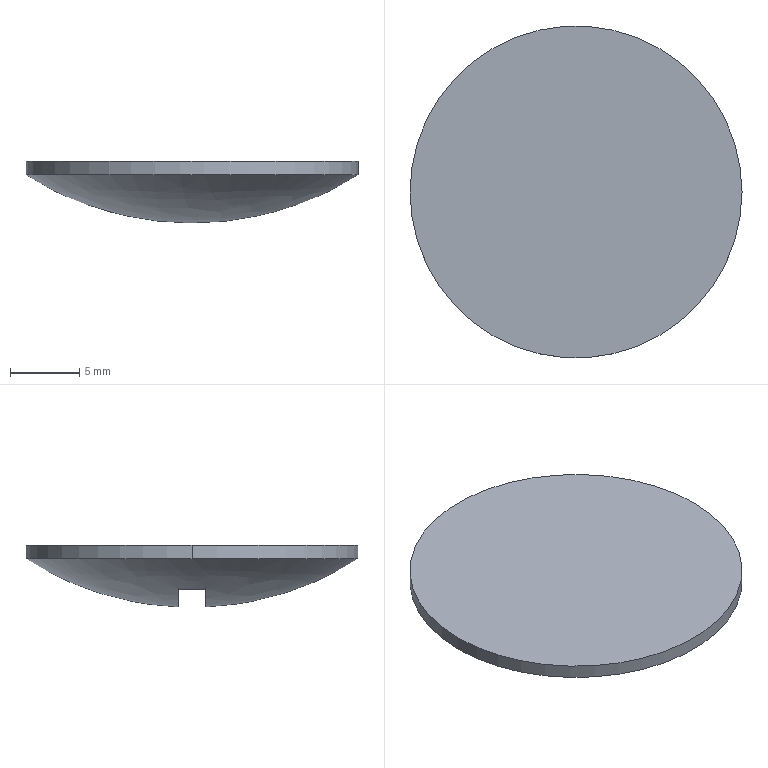Part | STEP file | PRODUCT_NAME_42_default | 1 solid | 9 faces | box 24 x 24 x 4.478 mm | volume 1175 mm3 | plane 6 | cylinder 2 | spline 1 | commonest cylinder face diameters 24 x2
STEP:
#1=CARTESIAN_POINT('',(0.,0.,0.));
#2=DIRECTION('',(0.,0.,1.));
#3=DIRECTION('',(1.,0.,0.));
#4=AXIS2_PLACEMENT_3D('',#1,#2,#3);
#5=CARTESIAN_POINT('',(194.5,-10.5,-47.5));
#6=VERTEX_POINT('',#5);
#7=CARTESIAN_POINT('',(170.5,-10.5,-47.5));
#8=VERTEX_POINT('',#7);
#9=CARTESIAN_POINT('',(182.5,-10.5,-47.5));
#10=DIRECTION('',(0.,0.,1.));
#11=DIRECTION('',(-1.,0.,0.));
#12=AXIS2_PLACEMENT_3D('',#9,#10,#11);
#13=CIRCLE('',#12,12.);
#14=CARTESIAN_POINT('',(182.5,-10.5,-48.));
#15=DIRECTION('',(0.,0.,-1.));
#16=DIRECTION('',(-1.,0.,0.));
#17=AXIS2_PLACEMENT_3D('',#14,#15,#16);
#18=CYLINDRICAL_SURFACE('',#17,12.);
#19=CARTESIAN_POINT('',(6.283,-0.5));
#20=DIRECTION('',(-1.,0.));
#21=VECTOR('',#20,1.);
#22=LINE('',#19,#21);
#23=(GEOMETRIC_REPRESENTATION_CONTEXT(2)PARAMETRIC_REPRESENTATION_CONTEXT()REPRESENTATION_CONTEXT('',''));
#24=DEFINITIONAL_REPRESENTATION('',(#22),#23);
#25=PCURVE('',#18,#24);
#26=CARTESIAN_POINT('',(188.5,-10.5,-47.5));
#27=DIRECTION('',(0.,0.,1.));
#28=DIRECTION('',(1.,0.,0.));
#29=AXIS2_PLACEMENT_3D('',#26,#27,#28);
#30=PLANE('',#29);
#31=CARTESIAN_POINT('',(-6.,0.));
#32=DIRECTION('',(-1.,0.));
#33=AXIS2_PLACEMENT_2D('',#31,#32);
#34=CIRCLE('',#33,12.);
#35=(GEOMETRIC_REPRESENTATION_CONTEXT(2)PARAMETRIC_REPRESENTATION_CONTEXT()REPRESENTATION_CONTEXT('',''));
#36=DEFINITIONAL_REPRESENTATION('',(#34),#35);
#37=PCURVE('',#30,#36);
#38=SURFACE_CURVE('',#13,(#25,#37),.PCURVE_S1.);
#39=EDGE_CURVE('',#6,#8,#38,.T.);
#40=ORIENTED_EDGE('',*,*,#39,.F.);
#41=CARTESIAN_POINT('',(194.5,-10.5,-48.5));
#42=VERTEX_POINT('',#41);
#43=CARTESIAN_POINT('',(194.5,-10.5,-48.));
#44=DIRECTION('',(0.,0.,-1.));
#45=VECTOR('',#44,1.);
#46=LINE('',#43,#45);
#47=CARTESIAN_POINT('',(3.142,0.));
#48=DIRECTION('',(0.,1.));
#49=VECTOR('',#48,1.);
#50=LINE('',#47,#49);
#51=(GEOMETRIC_REPRESENTATION_CONTEXT(2)PARAMETRIC_REPRESENTATION_CONTEXT()REPRESENTATION_CONTEXT('',''));
#52=DEFINITIONAL_REPRESENTATION('',(#50),#51);
#53=PCURVE('',#18,#52);
#54=CARTESIAN_POINT('',(182.5,-10.5,-48.));
#55=DIRECTION('',(0.,0.,-1.));
#56=DIRECTION('',(-1.,0.,0.));
#57=AXIS2_PLACEMENT_3D('',#54,#55,#56);
#58=CYLINDRICAL_SURFACE('',#57,12.);
#59=CARTESIAN_POINT('',(3.142,0.));
#60=DIRECTION('',(0.,1.));
#61=VECTOR('',#60,1.);
#62=LINE('',#59,#61);
#63=(GEOMETRIC_REPRESENTATION_CONTEXT(2)PARAMETRIC_REPRESENTATION_CONTEXT()REPRESENTATION_CONTEXT('',''));
#64=DEFINITIONAL_REPRESENTATION('',(#62),#63);
#65=PCURVE('',#58,#64);
#66=SURFACE_CURVE('',#46,(#53,#65),.PCURVE_S1.);
#67=EDGE_CURVE('',#6,#42,#66,.T.);
#68=ORIENTED_EDGE('',*,*,#67,.T.);
#69=CARTESIAN_POINT('',(170.5,-10.5,-48.5));
#70=VERTEX_POINT('',#69);
#71=CARTESIAN_POINT('',(182.5,-10.5,-48.5));
#72=DIRECTION('',(0.,0.,1.));
#73=DIRECTION('',(-1.,0.,0.));
#74=AXIS2_PLACEMENT_3D('',#71,#72,#73);
#75=CIRCLE('',#74,12.);
#76=CARTESIAN_POINT('',(6.283,0.5));
#77=DIRECTION('',(-1.,0.));
#78=VECTOR('',#77,1.);
#79=LINE('',#76,#78);
#80=(GEOMETRIC_REPRESENTATION_CONTEXT(2)PARAMETRIC_REPRESENTATION_CONTEXT()REPRESENTATION_CONTEXT('',''));
#81=DEFINITIONAL_REPRESENTATION('',(#79),#80);
#82=PCURVE('',#18,#81);
#83=CARTESIAN_POINT('',(194.7,-20.681,-45.355));
#84=CARTESIAN_POINT('',(194.7,-14.291,-49.505));
#85=CARTESIAN_POINT('',(194.7,-6.671,-49.498));
#86=CARTESIAN_POINT('',(194.7,-0.2882,-45.335));
#87=CARTESIAN_POINT('',(187.09,-23.387,-49.521));
#88=CARTESIAN_POINT('',(187.09,-15.298,-54.774));
#89=CARTESIAN_POINT('',(187.09,-5.653,-54.765));
#90=CARTESIAN_POINT('',(187.09,2.426,-49.495));
#91=CARTESIAN_POINT('',(178.001,-23.396,-49.535));
#92=CARTESIAN_POINT('',(178.001,-15.301,-54.793));
#93=CARTESIAN_POINT('',(178.001,-5.649,-54.783));
#94=CARTESIAN_POINT('',(178.001,2.435,-49.51));
#95=CARTESIAN_POINT('',(170.372,-20.706,-45.394));
#96=CARTESIAN_POINT('',(170.372,-14.3,-49.555));
#97=CARTESIAN_POINT('',(170.372,-6.661,-49.547));
#98=CARTESIAN_POINT('',(170.372,-0.2627,-45.374));
#99=(BOUNDED_SURFACE()B_SPLINE_SURFACE(3,3,((#83,#84,#85,#86),(#87,#88,#89,#90),(#91,#92,#93,#94),(#95,#96,#97,#98)),.UNSPECIFIED.,.F.,.F.,.F.)B_SPLINE_SURFACE_WITH_KNOTS((4,4),(4,4),(0.,1.),(0.,1.),.PIECEWISE_BEZIER_KNOTS.)GEOMETRIC_REPRESENTATION_ITEM()RATIONAL_B_SPLINE_SURFACE(((1.,0.8921,0.8921,1.),(0.8923,0.796,0.796,0.8923),(0.8923,0.796,0.796,0.8923),(1.,0.8921,0.8921,1.)))REPRESENTATION_ITEM('')SURFACE());
#100=CARTESIAN_POINT('',(0.009777,0.4992));
#101=CARTESIAN_POINT('',(0.009731,0.5248));
#102=CARTESIAN_POINT('',(0.01378,0.5759));
#103=CARTESIAN_POINT('',(0.03134,0.6501));
#104=CARTESIAN_POINT('',(0.05961,0.7196));
#105=CARTESIAN_POINT('',(0.09719,0.7826));
#106=CARTESIAN_POINT('',(0.1425,0.8381));
#107=CARTESIAN_POINT('',(0.1941,0.8853));
#108=CARTESIAN_POINT('',(0.2505,0.9239));
#109=CARTESIAN_POINT('',(0.3105,0.9538));
#110=CARTESIAN_POINT('',(0.3729,0.975));
#111=CARTESIAN_POINT('',(0.4369,0.9877));
#112=CARTESIAN_POINT('',(0.5016,0.9919));
#113=CARTESIAN_POINT('',(0.5664,0.9877));
#114=CARTESIAN_POINT('',(0.6304,0.975));
#115=CARTESIAN_POINT('',(0.6928,0.9538));
#116=CARTESIAN_POINT('',(0.7528,0.9239));
#117=CARTESIAN_POINT('',(0.8092,0.8853));
#118=CARTESIAN_POINT('',(0.8608,0.8381));
#119=CARTESIAN_POINT('',(0.9062,0.7826));
#120=CARTESIAN_POINT('',(0.9439,0.7196));
#121=CARTESIAN_POINT('',(0.9722,0.6501));
#122=CARTESIAN_POINT('',(0.9897,0.5759));
#123=CARTESIAN_POINT('',(0.9938,0.5248));
#124=CARTESIAN_POINT('',(0.9937,0.4992));
#125=B_SPLINE_CURVE_WITH_KNOTS('',3,(#100,#101,#102,#103,#104,#105,#106,#107,#108,#109,#110,#111,#112,#113,#114,#115,#116,#117,#118,#119,#120,#121,#122,#123,#124),.UNSPECIFIED.,.F.,.F.,(4,1,1,1,1,1,1,1,1,1,1,1,1,1,1,1,1,1,1,1,1,1,4),(3.142,3.284,3.427,3.57,3.713,3.856,3.998,4.141,4.284,4.427,4.57,4.712,4.855,4.998,5.141,5.284,5.426,5.569,5.712,5.855,5.998,6.14,6.283),.QUASI_UNIFORM_KNOTS.);
#126=(GEOMETRIC_REPRESENTATION_CONTEXT(2)PARAMETRIC_REPRESENTATION_CONTEXT()REPRESENTATION_CONTEXT('',''));
#127=DEFINITIONAL_REPRESENTATION('',(#125),#126);
#128=PCURVE('',#99,#127);
#129=SURFACE_CURVE('',#75,(#82,#128),.PCURVE_S1.);
#130=EDGE_CURVE('',#42,#70,#129,.T.);
#131=ORIENTED_EDGE('',*,*,#130,.T.);
#132=CARTESIAN_POINT('',(170.5,-10.5,-48.));
#133=DIRECTION('',(0.,0.,-1.));
#134=VECTOR('',#133,1.);
#135=LINE('',#132,#134);
#136=CARTESIAN_POINT('',(0.,0.));
#137=DIRECTION('',(0.,1.));
#138=VECTOR('',#137,1.);
#139=LINE('',#136,#138);
#140=(GEOMETRIC_REPRESENTATION_CONTEXT(2)PARAMETRIC_REPRESENTATION_CONTEXT()REPRESENTATION_CONTEXT('',''));
#141=DEFINITIONAL_REPRESENTATION('',(#139),#140);
#142=PCURVE('',#18,#141);
#143=CARTESIAN_POINT('',(6.283,0.));
#144=DIRECTION('',(0.,1.));
#145=VECTOR('',#144,1.);
#146=LINE('',#143,#145);
#147=(GEOMETRIC_REPRESENTATION_CONTEXT(2)PARAMETRIC_REPRESENTATION_CONTEXT()REPRESENTATION_CONTEXT('',''));
#148=DEFINITIONAL_REPRESENTATION('',(#146),#147);
#149=PCURVE('',#58,#148);
#150=SURFACE_CURVE('',#135,(#142,#149),.PCURVE_S1.);
#151=EDGE_CURVE('',#8,#70,#150,.T.);
#152=ORIENTED_EDGE('',*,*,#151,.F.);
#153=EDGE_LOOP('',(#40,#68,#131,#152));
#154=FACE_BOUND('',#153,.T.);
#155=ADVANCED_FACE('',(#154),#18,.T.);
#156=CARTESIAN_POINT('',(182.5,-10.5,-47.5));
#157=DIRECTION('',(0.,0.,1.));
#158=DIRECTION('',(-1.,0.,0.));
#159=AXIS2_PLACEMENT_3D('',#156,#157,#158);
#160=CIRCLE('',#159,12.);
#161=CARTESIAN_POINT('',(-6.,0.));
#162=DIRECTION('',(-1.,0.));
#163=AXIS2_PLACEMENT_2D('',#161,#162);
#164=CIRCLE('',#163,12.);
#165=(GEOMETRIC_REPRESENTATION_CONTEXT(2)PARAMETRIC_REPRESENTATION_CONTEXT()REPRESENTATION_CONTEXT('',''));
#166=DEFINITIONAL_REPRESENTATION('',(#164),#165);
#167=PCURVE('',#30,#166);
#168=CARTESIAN_POINT('',(6.283,-0.5));
#169=DIRECTION('',(-1.,0.));
#170=VECTOR('',#169,1.);
#171=LINE('',#168,#170);
#172=(GEOMETRIC_REPRESENTATION_CONTEXT(2)PARAMETRIC_REPRESENTATION_CONTEXT()REPRESENTATION_CONTEXT('',''));
#173=DEFINITIONAL_REPRESENTATION('',(#171),#172);
#174=PCURVE('',#58,#173);
#175=SURFACE_CURVE('',#160,(#167,#174),.PCURVE_S1.);
#176=EDGE_CURVE('',#8,#6,#175,.T.);
#177=ORIENTED_EDGE('',*,*,#176,.T.);
#178=ORIENTED_EDGE('',*,*,#39,.T.);
#179=EDGE_LOOP('',(#177,#178));
#180=FACE_BOUND('',#179,.T.);
#181=ADVANCED_FACE('',(#180),#30,.T.);
#182=ORIENTED_EDGE('',*,*,#67,.F.);
#183=ORIENTED_EDGE('',*,*,#176,.F.);
#184=ORIENTED_EDGE('',*,*,#151,.T.);
#185=CARTESIAN_POINT('',(182.5,-10.5,-48.5));
#186=DIRECTION('',(0.,0.,1.));
#187=DIRECTION('',(-1.,0.,0.));
#188=AXIS2_PLACEMENT_3D('',#185,#186,#187);
#189=CIRCLE('',#188,12.);
#190=CARTESIAN_POINT('',(6.283,0.5));
#191=DIRECTION('',(-1.,0.));
#192=VECTOR('',#191,1.);
#193=LINE('',#190,#192);
#194=(GEOMETRIC_REPRESENTATION_CONTEXT(2)PARAMETRIC_REPRESENTATION_CONTEXT()REPRESENTATION_CONTEXT('',''));
#195=DEFINITIONAL_REPRESENTATION('',(#193),#194);
#196=PCURVE('',#58,#195);
#197=CARTESIAN_POINT('',(0.9937,0.4992));
#198=CARTESIAN_POINT('',(0.9938,0.4736));
#199=CARTESIAN_POINT('',(0.9897,0.4225));
#200=CARTESIAN_POINT('',(0.9722,0.3483));
#201=CARTESIAN_POINT('',(0.9439,0.2788));
#202=CARTESIAN_POINT('',(0.9062,0.2157));
#203=CARTESIAN_POINT('',(0.8608,0.1602));
#204=CARTESIAN_POINT('',(0.8092,0.1129));
#205=CARTESIAN_POINT('',(0.7528,0.07436));
#206=CARTESIAN_POINT('',(0.6928,0.04446));
#207=CARTESIAN_POINT('',(0.6304,0.02321));
#208=CARTESIAN_POINT('',(0.5664,0.01051));
#209=CARTESIAN_POINT('',(0.5016,0.006284));
#210=CARTESIAN_POINT('',(0.4369,0.01051));
#211=CARTESIAN_POINT('',(0.3729,0.02321));
#212=CARTESIAN_POINT('',(0.3105,0.04446));
#213=CARTESIAN_POINT('',(0.2505,0.07436));
#214=CARTESIAN_POINT('',(0.1941,0.1129));
#215=CARTESIAN_POINT('',(0.1425,0.1602));
#216=CARTESIAN_POINT('',(0.09719,0.2157));
#217=CARTESIAN_POINT('',(0.05961,0.2788));
#218=CARTESIAN_POINT('',(0.03134,0.3483));
#219=CARTESIAN_POINT('',(0.01378,0.4225));
#220=CARTESIAN_POINT('',(0.009731,0.4736));
#221=CARTESIAN_POINT('',(0.009777,0.4992));
#222=B_SPLINE_CURVE_WITH_KNOTS('',3,(#197,#198,#199,#200,#201,#202,#203,#204,#205,#206,#207,#208,#209,#210,#211,#212,#213,#214,#215,#216,#217,#218,#219,#220,#221),.UNSPECIFIED.,.F.,.F.,(4,1,1,1,1,1,1,1,1,1,1,1,1,1,1,1,1,1,1,1,1,1,4),(0.,0.1428,0.2856,0.4284,0.5712,0.714,0.8568,0.9996,1.142,1.285,1.428,1.571,1.714,1.856,1.999,2.142,2.285,2.428,2.57,2.713,2.856,2.999,3.142),.QUASI_UNIFORM_KNOTS.);
#223=(GEOMETRIC_REPRESENTATION_CONTEXT(2)PARAMETRIC_REPRESENTATION_CONTEXT()REPRESENTATION_CONTEXT('',''));
#224=DEFINITIONAL_REPRESENTATION('',(#222),#223);
#225=PCURVE('',#99,#224);
#226=SURFACE_CURVE('',#189,(#196,#225),.PCURVE_S1.);
#227=EDGE_CURVE('',#70,#42,#226,.T.);
#228=ORIENTED_EDGE('',*,*,#227,.T.);
#229=EDGE_LOOP('',(#182,#183,#184,#228));
#230=FACE_BOUND('',#229,.T.);
#231=ADVANCED_FACE('',(#230),#58,.T.);
#232=CARTESIAN_POINT('',(175.,-11.5,-50.678));
#233=VERTEX_POINT('',#232);
#234=CARTESIAN_POINT('',(190.,-11.5,-50.678));
#235=VERTEX_POINT('',#234);
#236=CARTESIAN_POINT('',(175.,-11.5,-50.678));
#237=CARTESIAN_POINT('',(176.213,-11.5,-51.112));
#238=CARTESIAN_POINT('',(177.444,-11.5,-51.434));
#239=CARTESIAN_POINT('',(179.32,-11.5,-51.759));
#240=CARTESIAN_POINT('',(179.95,-11.5,-51.841));
#241=CARTESIAN_POINT('',(181.22,-11.5,-51.95));
#242=CARTESIAN_POINT('',(181.861,-11.5,-51.978));
#243=CARTESIAN_POINT('',(183.79,-11.5,-51.977));
#244=CARTESIAN_POINT('',(185.057,-11.5,-51.867));
#245=CARTESIAN_POINT('',(187.556,-11.5,-51.434));
#246=CARTESIAN_POINT('',(188.787,-11.5,-51.112));
#247=CARTESIAN_POINT('',(190.,-11.5,-50.678));
#248=B_SPLINE_CURVE_WITH_KNOTS('',3,(#236,#237,#238,#239,#240,#241,#242,#243,#244,#245,#246,#247),.UNSPECIFIED.,.F.,.F.,(4,2,2,2,2,4),(0.,0.003808,0.005712,0.007615,0.01142,0.01523),.UNSPECIFIED.);
#249=CARTESIAN_POINT('',(0.7935,0.4591));
#250=CARTESIAN_POINT('',(0.7844,0.4592));
#251=CARTESIAN_POINT('',(0.7663,0.4595));
#252=CARTESIAN_POINT('',(0.7394,0.4599));
#253=CARTESIAN_POINT('',(0.7126,0.4602));
#254=CARTESIAN_POINT('',(0.6861,0.4605));
#255=CARTESIAN_POINT('',(0.6596,0.4608));
#256=CARTESIAN_POINT('',(0.6333,0.461));
#257=CARTESIAN_POINT('',(0.607,0.4611));
#258=CARTESIAN_POINT('',(0.5807,0.4613));
#259=CARTESIAN_POINT('',(0.5544,0.4613));
#260=CARTESIAN_POINT('',(0.528,0.4614));
#261=CARTESIAN_POINT('',(0.5015,0.4614));
#262=CARTESIAN_POINT('',(0.475,0.4614));
#263=CARTESIAN_POINT('',(0.4487,0.4613));
#264=CARTESIAN_POINT('',(0.4224,0.4613));
#265=CARTESIAN_POINT('',(0.3962,0.4611));
#266=CARTESIAN_POINT('',(0.3699,0.461));
#267=CARTESIAN_POINT('',(0.3436,0.4607));
#268=CARTESIAN_POINT('',(0.3172,0.4605));
#269=CARTESIAN_POINT('',(0.2906,0.4602));
#270=CARTESIAN_POINT('',(0.2639,0.4599));
#271=CARTESIAN_POINT('',(0.237,0.4595));
#272=CARTESIAN_POINT('',(0.2189,0.4592));
#273=CARTESIAN_POINT('',(0.2098,0.4591));
#274=B_SPLINE_CURVE_WITH_KNOTS('',3,(#249,#250,#251,#252,#253,#254,#255,#256,#257,#258,#259,#260,#261,#262,#263,#264,#265,#266,#267,#268,#269,#270,#271,#272,#273),.UNSPECIFIED.,.F.,.F.,(4,1,1,1,1,1,1,1,1,1,1,1,1,1,1,1,1,1,1,1,1,1,4),(0.,0.0006923,0.001385,0.002077,0.002769,0.003462,0.004154,0.004846,0.005539,0.006231,0.006923,0.007615,0.008308,0.009,0.009692,0.01038,0.01108,0.01177,0.01246,0.01315,0.01385,0.01454,0.01523),.QUASI_UNIFORM_KNOTS.);
#275=(GEOMETRIC_REPRESENTATION_CONTEXT(2)PARAMETRIC_REPRESENTATION_CONTEXT()REPRESENTATION_CONTEXT('',''));
#276=DEFINITIONAL_REPRESENTATION('',(#274),#275);
#277=PCURVE('',#99,#276);
#278=CARTESIAN_POINT('',(182.5,-11.5,-50.75));
#279=DIRECTION('',(0.,1.,0.));
#280=DIRECTION('',(0.,0.,1.));
#281=AXIS2_PLACEMENT_3D('',#278,#279,#280);
#282=PLANE('',#281);
#283=CARTESIAN_POINT('',(0.07152,-7.5));
#284=CARTESIAN_POINT('',(-0.3615,-6.287));
#285=CARTESIAN_POINT('',(-0.684,-5.056));
#286=CARTESIAN_POINT('',(-1.009,-3.18));
#287=CARTESIAN_POINT('',(-1.091,-2.55));
#288=CARTESIAN_POINT('',(-1.2,-1.28));
#289=CARTESIAN_POINT('',(-1.228,-0.6394));
#290=CARTESIAN_POINT('',(-1.227,1.29));
#291=CARTESIAN_POINT('',(-1.117,2.557));
#292=CARTESIAN_POINT('',(-0.6838,5.056));
#293=CARTESIAN_POINT('',(-0.3615,6.287));
#294=CARTESIAN_POINT('',(0.07152,7.5));
#295=B_SPLINE_CURVE_WITH_KNOTS('',3,(#283,#284,#285,#286,#287,#288,#289,#290,#291,#292,#293,#294),.UNSPECIFIED.,.F.,.F.,(4,2,2,2,2,4),(0.,0.003808,0.005712,0.007615,0.01142,0.01523),.UNSPECIFIED.);
#296=(GEOMETRIC_REPRESENTATION_CONTEXT(2)PARAMETRIC_REPRESENTATION_CONTEXT()REPRESENTATION_CONTEXT('',''));
#297=DEFINITIONAL_REPRESENTATION('',(#295),#296);
#298=PCURVE('',#282,#297);
#299=SURFACE_CURVE('',#248,(#277,#298),.PCURVE_S1.);
#300=EDGE_CURVE('',#233,#235,#299,.T.);
#301=ORIENTED_EDGE('',*,*,#300,.T.);
#302=CARTESIAN_POINT('',(190.,-9.5,-50.678));
#303=VERTEX_POINT('',#302);
#304=CARTESIAN_POINT('',(190.,-10.5,-29.679));
#305=DIRECTION('',(-1.,0.,0.));
#306=DIRECTION('',(0.,0.,-1.));
#307=AXIS2_PLACEMENT_3D('',#304,#305,#306);
#308=CIRCLE('',#307,21.024);
#309=CARTESIAN_POINT('',(0.2098,0.5393));
#310=CARTESIAN_POINT('',(0.2098,0.538));
#311=CARTESIAN_POINT('',(0.2098,0.5356));
#312=CARTESIAN_POINT('',(0.2098,0.532));
#313=CARTESIAN_POINT('',(0.2098,0.5283));
#314=CARTESIAN_POINT('',(0.2098,0.5247));
#315=CARTESIAN_POINT('',(0.2098,0.521));
#316=CARTESIAN_POINT('',(0.2098,0.5174));
#317=CARTESIAN_POINT('',(0.2098,0.5137));
#318=CARTESIAN_POINT('',(0.2098,0.5101));
#319=CARTESIAN_POINT('',(0.2098,0.5065));
#320=CARTESIAN_POINT('',(0.2098,0.5028));
#321=CARTESIAN_POINT('',(0.2098,0.4992));
#322=CARTESIAN_POINT('',(0.2098,0.4955));
#323=CARTESIAN_POINT('',(0.2098,0.4919));
#324=CARTESIAN_POINT('',(0.2098,0.4882));
#325=CARTESIAN_POINT('',(0.2098,0.4846));
#326=CARTESIAN_POINT('',(0.2098,0.481));
#327=CARTESIAN_POINT('',(0.2098,0.4773));
#328=CARTESIAN_POINT('',(0.2098,0.4737));
#329=CARTESIAN_POINT('',(0.2098,0.47));
#330=CARTESIAN_POINT('',(0.2098,0.4664));
#331=CARTESIAN_POINT('',(0.2098,0.4627));
#332=CARTESIAN_POINT('',(0.2098,0.4603));
#333=CARTESIAN_POINT('',(0.2098,0.4591));
#334=B_SPLINE_CURVE_WITH_KNOTS('',3,(#309,#310,#311,#312,#313,#314,#315,#316,#317,#318,#319,#320,#321,#322,#323,#324,#325,#326,#327,#328,#329,#330,#331,#332,#333),.UNSPECIFIED.,.F.,.F.,(4,1,1,1,1,1,1,1,1,1,1,1,1,1,1,1,1,1,1,1,1,1,4),(6.236,6.24,6.244,6.249,6.253,6.257,6.262,6.266,6.27,6.275,6.279,6.283,6.288,6.292,6.296,6.3,6.305,6.309,6.313,6.318,6.322,6.326,6.331),.QUASI_UNIFORM_KNOTS.);
#335=(GEOMETRIC_REPRESENTATION_CONTEXT(2)PARAMETRIC_REPRESENTATION_CONTEXT()REPRESENTATION_CONTEXT('',''));
#336=DEFINITIONAL_REPRESENTATION('',(#334),#335);
#337=PCURVE('',#99,#336);
#338=CARTESIAN_POINT('',(190.,-10.5,-50.75));
#339=DIRECTION('',(-1.,0.,0.));
#340=DIRECTION('',(0.,0.,1.));
#341=AXIS2_PLACEMENT_3D('',#338,#339,#340);
#342=PLANE('',#341);
#343=CARTESIAN_POINT('',(21.071,0.));
#344=DIRECTION('',(-1.,0.));
#345=AXIS2_PLACEMENT_2D('',#343,#344);
#346=CIRCLE('',#345,21.024);
#347=(GEOMETRIC_REPRESENTATION_CONTEXT(2)PARAMETRIC_REPRESENTATION_CONTEXT()REPRESENTATION_CONTEXT('',''));
#348=DEFINITIONAL_REPRESENTATION('',(#346),#347);
#349=PCURVE('',#342,#348);
#350=SURFACE_CURVE('',#308,(#337,#349),.PCURVE_S1.);
#351=EDGE_CURVE('',#303,#235,#350,.T.);
#352=ORIENTED_EDGE('',*,*,#351,.F.);
#353=CARTESIAN_POINT('',(175.,-9.5,-50.678));
#354=VERTEX_POINT('',#353);
#355=CARTESIAN_POINT('',(190.,-9.5,-50.678));
#356=CARTESIAN_POINT('',(188.787,-9.5,-51.112));
#357=CARTESIAN_POINT('',(187.556,-9.5,-51.434));
#358=CARTESIAN_POINT('',(185.68,-9.5,-51.759));
#359=CARTESIAN_POINT('',(185.05,-9.5,-51.841));
#360=CARTESIAN_POINT('',(183.78,-9.5,-51.95));
#361=CARTESIAN_POINT('',(183.139,-9.5,-51.978));
#362=CARTESIAN_POINT('',(181.21,-9.5,-51.977));
#363=CARTESIAN_POINT('',(179.943,-9.5,-51.867));
#364=CARTESIAN_POINT('',(177.444,-9.5,-51.434));
#365=CARTESIAN_POINT('',(176.213,-9.5,-51.112));
#366=CARTESIAN_POINT('',(175.,-9.5,-50.678));
#367=B_SPLINE_CURVE_WITH_KNOTS('',3,(#355,#356,#357,#358,#359,#360,#361,#362,#363,#364,#365,#366),.UNSPECIFIED.,.F.,.F.,(4,2,2,2,2,4),(0.,0.003808,0.005712,0.007615,0.01142,0.01523),.UNSPECIFIED.);
#368=CARTESIAN_POINT('',(0.2098,0.5393));
#369=CARTESIAN_POINT('',(0.2189,0.5391));
#370=CARTESIAN_POINT('',(0.237,0.5388));
#371=CARTESIAN_POINT('',(0.2639,0.5385));
#372=CARTESIAN_POINT('',(0.2907,0.5381));
#373=CARTESIAN_POINT('',(0.3172,0.5378));
#374=CARTESIAN_POINT('',(0.3436,0.5376));
#375=CARTESIAN_POINT('',(0.37,0.5374));
#376=CARTESIAN_POINT('',(0.3963,0.5372));
#377=CARTESIAN_POINT('',(0.4226,0.5371));
#378=CARTESIAN_POINT('',(0.4489,0.537));
#379=CARTESIAN_POINT('',(0.4753,0.5369));
#380=CARTESIAN_POINT('',(0.5018,0.5369));
#381=CARTESIAN_POINT('',(0.5282,0.5369));
#382=CARTESIAN_POINT('',(0.5546,0.537));
#383=CARTESIAN_POINT('',(0.5808,0.5371));
#384=CARTESIAN_POINT('',(0.6071,0.5372));
#385=CARTESIAN_POINT('',(0.6334,0.5374));
#386=CARTESIAN_POINT('',(0.6597,0.5376));
#387=CARTESIAN_POINT('',(0.6861,0.5378));
#388=CARTESIAN_POINT('',(0.7126,0.5381));
#389=CARTESIAN_POINT('',(0.7394,0.5385));
#390=CARTESIAN_POINT('',(0.7663,0.5388));
#391=CARTESIAN_POINT('',(0.7844,0.5391));
#392=CARTESIAN_POINT('',(0.7935,0.5393));
#393=B_SPLINE_CURVE_WITH_KNOTS('',3,(#368,#369,#370,#371,#372,#373,#374,#375,#376,#377,#378,#379,#380,#381,#382,#383,#384,#385,#386,#387,#388,#389,#390,#391,#392),.UNSPECIFIED.,.F.,.F.,(4,1,1,1,1,1,1,1,1,1,1,1,1,1,1,1,1,1,1,1,1,1,4),(0.,0.0006923,0.001385,0.002077,0.002769,0.003462,0.004154,0.004846,0.005539,0.006231,0.006923,0.007615,0.008308,0.009,0.009692,0.01038,0.01108,0.01177,0.01246,0.01315,0.01385,0.01454,0.01523),.QUASI_UNIFORM_KNOTS.);
#394=(GEOMETRIC_REPRESENTATION_CONTEXT(2)PARAMETRIC_REPRESENTATION_CONTEXT()REPRESENTATION_CONTEXT('',''));
#395=DEFINITIONAL_REPRESENTATION('',(#393),#394);
#396=PCURVE('',#99,#395);
#397=CARTESIAN_POINT('',(182.5,-9.5,-50.75));
#398=DIRECTION('',(0.,-1.,0.));
#399=DIRECTION('',(0.,0.,-1.));
#400=AXIS2_PLACEMENT_3D('',#397,#398,#399);
#401=PLANE('',#400);
#402=CARTESIAN_POINT('',(-0.07152,7.5));
#403=CARTESIAN_POINT('',(0.3615,6.287));
#404=CARTESIAN_POINT('',(0.684,5.056));
#405=CARTESIAN_POINT('',(1.009,3.18));
#406=CARTESIAN_POINT('',(1.091,2.55));
#407=CARTESIAN_POINT('',(1.2,1.28));
#408=CARTESIAN_POINT('',(1.228,0.6394));
#409=CARTESIAN_POINT('',(1.227,-1.29));
#410=CARTESIAN_POINT('',(1.117,-2.557));
#411=CARTESIAN_POINT('',(0.6838,-5.056));
#412=CARTESIAN_POINT('',(0.3615,-6.287));
#413=CARTESIAN_POINT('',(-0.07152,-7.5));
#414=B_SPLINE_CURVE_WITH_KNOTS('',3,(#402,#403,#404,#405,#406,#407,#408,#409,#410,#411,#412,#413),.UNSPECIFIED.,.F.,.F.,(4,2,2,2,2,4),(0.,0.003808,0.005712,0.007615,0.01142,0.01523),.UNSPECIFIED.);
#415=(GEOMETRIC_REPRESENTATION_CONTEXT(2)PARAMETRIC_REPRESENTATION_CONTEXT()REPRESENTATION_CONTEXT('',''));
#416=DEFINITIONAL_REPRESENTATION('',(#414),#415);
#417=PCURVE('',#401,#416);
#418=SURFACE_CURVE('',#367,(#396,#417),.PCURVE_S1.);
#419=EDGE_CURVE('',#303,#354,#418,.T.);
#420=ORIENTED_EDGE('',*,*,#419,.T.);
#421=CARTESIAN_POINT('',(175.,-10.5,-29.679));
#422=DIRECTION('',(1.,0.,0.));
#423=DIRECTION('',(0.,0.,-1.));
#424=AXIS2_PLACEMENT_3D('',#421,#422,#423);
#425=CIRCLE('',#424,21.024);
#426=CARTESIAN_POINT('',(0.7935,0.4591));
#427=CARTESIAN_POINT('',(0.7935,0.4603));
#428=CARTESIAN_POINT('',(0.7935,0.4627));
#429=CARTESIAN_POINT('',(0.7935,0.4664));
#430=CARTESIAN_POINT('',(0.7935,0.47));
#431=CARTESIAN_POINT('',(0.7935,0.4737));
#432=CARTESIAN_POINT('',(0.7935,0.4773));
#433=CARTESIAN_POINT('',(0.7935,0.481));
#434=CARTESIAN_POINT('',(0.7935,0.4846));
#435=CARTESIAN_POINT('',(0.7935,0.4882));
#436=CARTESIAN_POINT('',(0.7935,0.4919));
#437=CARTESIAN_POINT('',(0.7935,0.4955));
#438=CARTESIAN_POINT('',(0.7935,0.4992));
#439=CARTESIAN_POINT('',(0.7935,0.5028));
#440=CARTESIAN_POINT('',(0.7935,0.5065));
#441=CARTESIAN_POINT('',(0.7935,0.5101));
#442=CARTESIAN_POINT('',(0.7935,0.5137));
#443=CARTESIAN_POINT('',(0.7935,0.5174));
#444=CARTESIAN_POINT('',(0.7935,0.521));
#445=CARTESIAN_POINT('',(0.7935,0.5247));
#446=CARTESIAN_POINT('',(0.7935,0.5283));
#447=CARTESIAN_POINT('',(0.7935,0.532));
#448=CARTESIAN_POINT('',(0.7935,0.5356));
#449=CARTESIAN_POINT('',(0.7935,0.538));
#450=CARTESIAN_POINT('',(0.7935,0.5393));
#451=B_SPLINE_CURVE_WITH_KNOTS('',3,(#426,#427,#428,#429,#430,#431,#432,#433,#434,#435,#436,#437,#438,#439,#440,#441,#442,#443,#444,#445,#446,#447,#448,#449,#450),.UNSPECIFIED.,.F.,.F.,(4,1,1,1,1,1,1,1,1,1,1,1,1,1,1,1,1,1,1,1,1,1,4),(6.236,6.24,6.244,6.249,6.253,6.257,6.262,6.266,6.27,6.275,6.279,6.283,6.288,6.292,6.296,6.3,6.305,6.309,6.313,6.318,6.322,6.326,6.331),.QUASI_UNIFORM_KNOTS.);
#452=(GEOMETRIC_REPRESENTATION_CONTEXT(2)PARAMETRIC_REPRESENTATION_CONTEXT()REPRESENTATION_CONTEXT('',''));
#453=DEFINITIONAL_REPRESENTATION('',(#451),#452);
#454=PCURVE('',#99,#453);
#455=CARTESIAN_POINT('',(175.,-10.5,-50.75));
#456=DIRECTION('',(1.,0.,0.));
#457=DIRECTION('',(0.,0.,-1.));
#458=AXIS2_PLACEMENT_3D('',#455,#456,#457);
#459=PLANE('',#458);
#460=CARTESIAN_POINT('',(-21.071,0.));
#461=DIRECTION('',(1.,0.));
#462=AXIS2_PLACEMENT_2D('',#460,#461);
#463=CIRCLE('',#462,21.024);
#464=(GEOMETRIC_REPRESENTATION_CONTEXT(2)PARAMETRIC_REPRESENTATION_CONTEXT()REPRESENTATION_CONTEXT('',''));
#465=DEFINITIONAL_REPRESENTATION('',(#463),#464);
#466=PCURVE('',#459,#465);
#467=SURFACE_CURVE('',#425,(#454,#466),.PCURVE_S1.);
#468=EDGE_CURVE('',#233,#354,#467,.T.);
#469=ORIENTED_EDGE('',*,*,#468,.F.);
#470=EDGE_LOOP('',(#301,#352,#420,#469));
#471=FACE_BOUND('',#470,.T.);
#472=ORIENTED_EDGE('',*,*,#227,.F.);
#473=ORIENTED_EDGE('',*,*,#130,.F.);
#474=EDGE_LOOP('',(#472,#473));
#475=FACE_BOUND('',#474,.T.);
#476=ADVANCED_FACE('',(#471,#475),#99,.T.);
#477=CARTESIAN_POINT('',(190.,-9.5,-48.5));
#478=VERTEX_POINT('',#477);
#479=CARTESIAN_POINT('',(175.,-9.5,-48.5));
#480=VERTEX_POINT('',#479);
#481=CARTESIAN_POINT('',(182.5,-9.5,-48.5));
#482=DIRECTION('',(-1.,0.,0.));
#483=VECTOR('',#482,1.);
#484=LINE('',#481,#483);
#485=CARTESIAN_POINT('',(-2.25,0.));
#486=DIRECTION('',(0.,-1.));
#487=VECTOR('',#486,1.);
#488=LINE('',#485,#487);
#489=(GEOMETRIC_REPRESENTATION_CONTEXT(2)PARAMETRIC_REPRESENTATION_CONTEXT()REPRESENTATION_CONTEXT('',''));
#490=DEFINITIONAL_REPRESENTATION('',(#488),#489);
#491=PCURVE('',#401,#490);
#492=CARTESIAN_POINT('',(182.5,-10.5,-48.5));
#493=DIRECTION('',(0.,0.,-1.));
#494=DIRECTION('',(-1.,0.,0.));
#495=AXIS2_PLACEMENT_3D('',#492,#493,#494);
#496=PLANE('',#495);
#497=CARTESIAN_POINT('',(0.,1.));
#498=DIRECTION('',(1.,0.));
#499=VECTOR('',#498,1.);
#500=LINE('',#497,#499);
#501=(GEOMETRIC_REPRESENTATION_CONTEXT(2)PARAMETRIC_REPRESENTATION_CONTEXT()REPRESENTATION_CONTEXT('',''));
#502=DEFINITIONAL_REPRESENTATION('',(#500),#501);
#503=PCURVE('',#496,#502);
#504=SURFACE_CURVE('',#484,(#491,#503),.PCURVE_S1.);
#505=EDGE_CURVE('',#478,#480,#504,.T.);
#506=ORIENTED_EDGE('',*,*,#505,.T.);
#507=CARTESIAN_POINT('',(175.,-9.5,-50.75));
#508=DIRECTION('',(0.,0.,-1.));
#509=VECTOR('',#508,1.);
#510=LINE('',#507,#509);
#511=CARTESIAN_POINT('',(0.,-7.5));
#512=DIRECTION('',(1.,0.));
#513=VECTOR('',#512,1.);
#514=LINE('',#511,#513);
#515=(GEOMETRIC_REPRESENTATION_CONTEXT(2)PARAMETRIC_REPRESENTATION_CONTEXT()REPRESENTATION_CONTEXT('',''));
#516=DEFINITIONAL_REPRESENTATION('',(#514),#515);
#517=PCURVE('',#401,#516);
#518=CARTESIAN_POINT('',(0.,1.));
#519=DIRECTION('',(1.,0.));
#520=VECTOR('',#519,1.);
#521=LINE('',#518,#520);
#522=(GEOMETRIC_REPRESENTATION_CONTEXT(2)PARAMETRIC_REPRESENTATION_CONTEXT()REPRESENTATION_CONTEXT('',''));
#523=DEFINITIONAL_REPRESENTATION('',(#521),#522);
#524=PCURVE('',#459,#523);
#525=SURFACE_CURVE('',#510,(#517,#524),.PCURVE_S1.);
#526=EDGE_CURVE('',#480,#354,#525,.T.);
#527=ORIENTED_EDGE('',*,*,#526,.T.);
#528=ORIENTED_EDGE('',*,*,#419,.F.);
#529=CARTESIAN_POINT('',(190.,-9.5,-50.75));
#530=DIRECTION('',(0.,0.,1.));
#531=VECTOR('',#530,1.);
#532=LINE('',#529,#531);
#533=CARTESIAN_POINT('',(0.,7.5));
#534=DIRECTION('',(-1.,0.));
#535=VECTOR('',#534,1.);
#536=LINE('',#533,#535);
#537=(GEOMETRIC_REPRESENTATION_CONTEXT(2)PARAMETRIC_REPRESENTATION_CONTEXT()REPRESENTATION_CONTEXT('',''));
#538=DEFINITIONAL_REPRESENTATION('',(#536),#537);
#539=PCURVE('',#401,#538);
#540=CARTESIAN_POINT('',(0.,1.));
#541=DIRECTION('',(1.,0.));
#542=VECTOR('',#541,1.);
#543=LINE('',#540,#542);
#544=(GEOMETRIC_REPRESENTATION_CONTEXT(2)PARAMETRIC_REPRESENTATION_CONTEXT()REPRESENTATION_CONTEXT('',''));
#545=DEFINITIONAL_REPRESENTATION('',(#543),#544);
#546=PCURVE('',#342,#545);
#547=SURFACE_CURVE('',#532,(#539,#546),.PCURVE_S1.);
#548=EDGE_CURVE('',#303,#478,#547,.T.);
#549=ORIENTED_EDGE('',*,*,#548,.T.);
#550=EDGE_LOOP('',(#506,#527,#528,#549));
#551=FACE_BOUND('',#550,.T.);
#552=ADVANCED_FACE('',(#551),#401,.T.);
#553=CARTESIAN_POINT('',(175.,-11.5,-48.5));
#554=VERTEX_POINT('',#553);
#555=CARTESIAN_POINT('',(190.,-11.5,-48.5));
#556=VERTEX_POINT('',#555);
#557=CARTESIAN_POINT('',(182.5,-11.5,-48.5));
#558=DIRECTION('',(1.,0.,0.));
#559=VECTOR('',#558,1.);
#560=LINE('',#557,#559);
#561=CARTESIAN_POINT('',(2.25,0.));
#562=DIRECTION('',(0.,1.));
#563=VECTOR('',#562,1.);
#564=LINE('',#561,#563);
#565=(GEOMETRIC_REPRESENTATION_CONTEXT(2)PARAMETRIC_REPRESENTATION_CONTEXT()REPRESENTATION_CONTEXT('',''));
#566=DEFINITIONAL_REPRESENTATION('',(#564),#565);
#567=PCURVE('',#282,#566);
#568=CARTESIAN_POINT('',(0.,-1.));
#569=DIRECTION('',(-1.,0.));
#570=VECTOR('',#569,1.);
#571=LINE('',#568,#570);
#572=(GEOMETRIC_REPRESENTATION_CONTEXT(2)PARAMETRIC_REPRESENTATION_CONTEXT()REPRESENTATION_CONTEXT('',''));
#573=DEFINITIONAL_REPRESENTATION('',(#571),#572);
#574=PCURVE('',#496,#573);
#575=SURFACE_CURVE('',#560,(#567,#574),.PCURVE_S1.);
#576=EDGE_CURVE('',#554,#556,#575,.T.);
#577=ORIENTED_EDGE('',*,*,#576,.T.);
#578=CARTESIAN_POINT('',(190.,-11.5,-50.75));
#579=DIRECTION('',(0.,0.,-1.));
#580=VECTOR('',#579,1.);
#581=LINE('',#578,#580);
#582=CARTESIAN_POINT('',(0.,7.5));
#583=DIRECTION('',(-1.,0.));
#584=VECTOR('',#583,1.);
#585=LINE('',#582,#584);
#586=(GEOMETRIC_REPRESENTATION_CONTEXT(2)PARAMETRIC_REPRESENTATION_CONTEXT()REPRESENTATION_CONTEXT('',''));
#587=DEFINITIONAL_REPRESENTATION('',(#585),#586);
#588=PCURVE('',#282,#587);
#589=CARTESIAN_POINT('',(0.,-1.));
#590=DIRECTION('',(-1.,0.));
#591=VECTOR('',#590,1.);
#592=LINE('',#589,#591);
#593=(GEOMETRIC_REPRESENTATION_CONTEXT(2)PARAMETRIC_REPRESENTATION_CONTEXT()REPRESENTATION_CONTEXT('',''));
#594=DEFINITIONAL_REPRESENTATION('',(#592),#593);
#595=PCURVE('',#342,#594);
#596=SURFACE_CURVE('',#581,(#588,#595),.PCURVE_S1.);
#597=EDGE_CURVE('',#556,#235,#596,.T.);
#598=ORIENTED_EDGE('',*,*,#597,.T.);
#599=ORIENTED_EDGE('',*,*,#300,.F.);
#600=CARTESIAN_POINT('',(175.,-11.5,-50.75));
#601=DIRECTION('',(0.,0.,1.));
#602=VECTOR('',#601,1.);
#603=LINE('',#600,#602);
#604=CARTESIAN_POINT('',(0.,-7.5));
#605=DIRECTION('',(1.,0.));
#606=VECTOR('',#605,1.);
#607=LINE('',#604,#606);
#608=(GEOMETRIC_REPRESENTATION_CONTEXT(2)PARAMETRIC_REPRESENTATION_CONTEXT()REPRESENTATION_CONTEXT('',''));
#609=DEFINITIONAL_REPRESENTATION('',(#607),#608);
#610=PCURVE('',#282,#609);
#611=CARTESIAN_POINT('',(0.,-1.));
#612=DIRECTION('',(-1.,0.));
#613=VECTOR('',#612,1.);
#614=LINE('',#611,#613);
#615=(GEOMETRIC_REPRESENTATION_CONTEXT(2)PARAMETRIC_REPRESENTATION_CONTEXT()REPRESENTATION_CONTEXT('',''));
#616=DEFINITIONAL_REPRESENTATION('',(#614),#615);
#617=PCURVE('',#459,#616);
#618=SURFACE_CURVE('',#603,(#610,#617),.PCURVE_S1.);
#619=EDGE_CURVE('',#233,#554,#618,.T.);
#620=ORIENTED_EDGE('',*,*,#619,.T.);
#621=EDGE_LOOP('',(#577,#598,#599,#620));
#622=FACE_BOUND('',#621,.T.);
#623=ADVANCED_FACE('',(#622),#282,.T.);
#624=ORIENTED_EDGE('',*,*,#619,.F.);
#625=ORIENTED_EDGE('',*,*,#468,.T.);
#626=ORIENTED_EDGE('',*,*,#526,.F.);
#627=CARTESIAN_POINT('',(175.,-10.5,-48.5));
#628=DIRECTION('',(0.,-1.,0.));
#629=VECTOR('',#628,1.);
#630=LINE('',#627,#629);
#631=CARTESIAN_POINT('',(-2.25,0.));
#632=DIRECTION('',(0.,-1.));
#633=VECTOR('',#632,1.);
#634=LINE('',#631,#633);
#635=(GEOMETRIC_REPRESENTATION_CONTEXT(2)PARAMETRIC_REPRESENTATION_CONTEXT()REPRESENTATION_CONTEXT('',''));
#636=DEFINITIONAL_REPRESENTATION('',(#634),#635);
#637=PCURVE('',#459,#636);
#638=CARTESIAN_POINT('',(7.5,0.));
#639=DIRECTION('',(0.,-1.));
#640=VECTOR('',#639,1.);
#641=LINE('',#638,#640);
#642=(GEOMETRIC_REPRESENTATION_CONTEXT(2)PARAMETRIC_REPRESENTATION_CONTEXT()REPRESENTATION_CONTEXT('',''));
#643=DEFINITIONAL_REPRESENTATION('',(#641),#642);
#644=PCURVE('',#496,#643);
#645=SURFACE_CURVE('',#630,(#637,#644),.PCURVE_S1.);
#646=EDGE_CURVE('',#480,#554,#645,.T.);
#647=ORIENTED_EDGE('',*,*,#646,.T.);
#648=EDGE_LOOP('',(#624,#625,#626,#647));
#649=FACE_BOUND('',#648,.T.);
#650=ADVANCED_FACE('',(#649),#459,.T.);
#651=ORIENTED_EDGE('',*,*,#646,.F.);
#652=ORIENTED_EDGE('',*,*,#505,.F.);
#653=CARTESIAN_POINT('',(190.,-10.5,-48.5));
#654=DIRECTION('',(0.,-1.,0.));
#655=VECTOR('',#654,1.);
#656=LINE('',#653,#655);
#657=CARTESIAN_POINT('',(-7.5,0.));
#658=DIRECTION('',(0.,-1.));
#659=VECTOR('',#658,1.);
#660=LINE('',#657,#659);
#661=(GEOMETRIC_REPRESENTATION_CONTEXT(2)PARAMETRIC_REPRESENTATION_CONTEXT()REPRESENTATION_CONTEXT('',''));
#662=DEFINITIONAL_REPRESENTATION('',(#660),#661);
#663=PCURVE('',#496,#662);
#664=CARTESIAN_POINT('',(2.25,0.));
#665=DIRECTION('',(0.,-1.));
#666=VECTOR('',#665,1.);
#667=LINE('',#664,#666);
#668=(GEOMETRIC_REPRESENTATION_CONTEXT(2)PARAMETRIC_REPRESENTATION_CONTEXT()REPRESENTATION_CONTEXT('',''));
#669=DEFINITIONAL_REPRESENTATION('',(#667),#668);
#670=PCURVE('',#342,#669);
#671=SURFACE_CURVE('',#656,(#663,#670),.PCURVE_S1.);
#672=EDGE_CURVE('',#478,#556,#671,.T.);
#673=ORIENTED_EDGE('',*,*,#672,.T.);
#674=ORIENTED_EDGE('',*,*,#576,.F.);
#675=EDGE_LOOP('',(#651,#652,#673,#674));
#676=FACE_BOUND('',#675,.T.);
#677=ADVANCED_FACE('',(#676),#496,.T.);
#678=ORIENTED_EDGE('',*,*,#548,.F.);
#679=ORIENTED_EDGE('',*,*,#351,.T.);
#680=ORIENTED_EDGE('',*,*,#597,.F.);
#681=ORIENTED_EDGE('',*,*,#672,.F.);
#682=EDGE_LOOP('',(#678,#679,#680,#681));
#683=FACE_BOUND('',#682,.T.);
#684=ADVANCED_FACE('',(#683),#342,.T.);
#685=CLOSED_SHELL('',(#155,#181,#231,#476,#552,#623,#650,#677,#684));
#686=MANIFOLD_SOLID_BREP('',#685);
#687=(LENGTH_UNIT()NAMED_UNIT(*)SI_UNIT(.MILLI.,.METRE.));
#688=UNCERTAINTY_MEASURE_WITH_UNIT(LENGTH_MEASURE(0.00005),#687,'','');
#689=(NAMED_UNIT(*)PLANE_ANGLE_UNIT()SI_UNIT($,.RADIAN.));
#690=(NAMED_UNIT(*)SI_UNIT($,.STERADIAN.)SOLID_ANGLE_UNIT());
#691=(GEOMETRIC_REPRESENTATION_CONTEXT(3)GLOBAL_UNCERTAINTY_ASSIGNED_CONTEXT((#688))GLOBAL_UNIT_ASSIGNED_CONTEXT((#687,#689,#690))REPRESENTATION_CONTEXT('',''));
#692=ADVANCED_BREP_SHAPE_REPRESENTATION('',(#4,#686),#691);